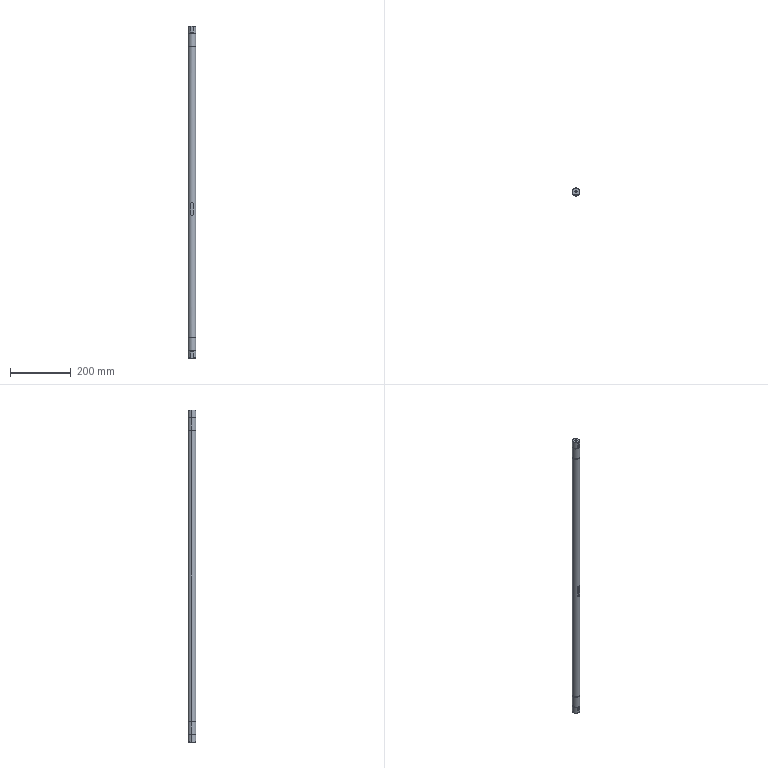Part | SolidWorks | features BaseBody 1 | 1 solid | 57 faces | box 25 x 25 x 1097 mm | volume 534043 mm3 | cylinder 28 | plane 19 | cone 10 | commonest cylinder face diameters 25 x10 23.9 x8 8 x6 6.8 x4